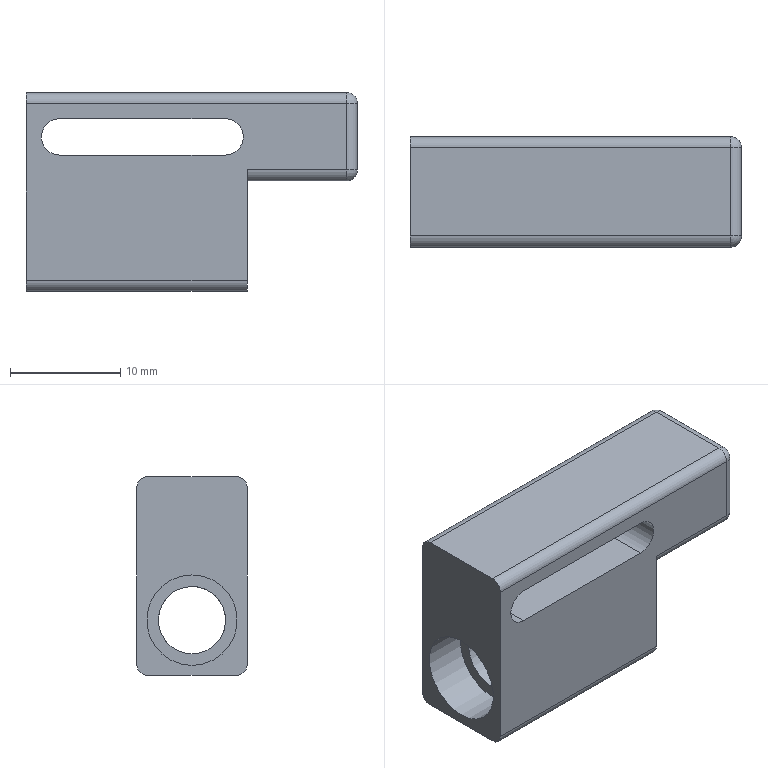CAM job | NX | 3+2 milling, drilling | part box 30 x 10 x 18 mm | stock box 35 x 12 x 23 mm
Tools:
number,name,description,diameter,corner_radius,flute_length,length,flutes
4,D4,平底铣刀-粗,4.0,0.0,25.0,75.0,2
9,D10,平底铣刀-粗,10.0,0.0,35.0,75.0,2
18,D4-J,平底铣刀-精,4.0,0.0,50.0,75.0,2
10,D10-J,平底铣刀-精,10.0,0.0,35.0,75.0,2
19,D6R0.5,圆鼻刀-粗,6.0,0.5,50.0,75.0,2
1,D80R0.8飞刀,圆鼻刀-粗,80.0,0.8,50.0,75.0,2
2,D6倒角刀,倒角刀,6.0,0.0,3.0,25.0,2
17,ZT6,钻头,6.0,0.0,35.0,50.0,2
Operations:
program,operation,operation_type,tool,method,geometry_group,spindle_rpm,surface_speed,feed_per_tooth,feed_cut,feed_plunge,cut_length_mm,path_length_mm,cut_time_min,machine_time_min
B,底壁铣飞面一刀开粗_COPY,VolumeBased25DMillingOperation,D10,分层开粗-切深K-步距G,W-B,7000.0,219.911,0.2143,3000.0,100.0,807.18,888.751,0.2691,0.2772
B,底壁铣分层开粗-中_COPY,VolumeBased25DMillingOperation,D10,分层开粗-切深K-步距G,W-B,7000.0,219.911,0.2857,4000.0,100.0,1176.861,1411.293,0.2942,0.3177
B,等高螺旋爬面_COPY,ZLevelMilling,D6R0.5,等高爬面-切深K-步距G,W-B,7000.0,175.929,0.3214,4500.0,100.0,1234.874,1273.374,0.2744,0.2783
B,平面去毛刺6X45L_COPY,SurfaceContour,D6倒角刀,爬面_倒角-切深0-步距G,W-B,6500.0,122.519,0.1154,1500.0,100.0,78.519,133.831,0.0523,0.0579
B,底壁铣飞面一刀精光_COPY,VolumeBased25DMillingOperation,D10-J,侧刃精光-切深K-步距G,W-B,7000.0,219.911,0.0714,1000.0,100.0,89.149,125.149,0.0891,0.0927
B,底壁铣精光底面-中_COPY,VolumeBased25DMillingOperation,D10-J,精光步距切深关,W-B,8000.0,251.32,0.0625,1000.0,100.0,49.923,96.523,0.0499,0.0546
B,底壁铣精光侧面-中-选底面_COPY_1,VolumeBased25DMillingOperation,D10-J,侧刃精光-切深K-步距G,W-B,8000.0,251.32,0.0625,1000.0,100.0,35.035,82.635,0.035,0.0398
A,顶面,FaceMilling,D80R0.8飞刀,侧刃精光-切深K-步距G,W-A,5000.0,1256.637,0.1,1000.0,100.0,112.0,148.0,0.112,0.1156
A,外形粗_2,VolumeBased25DMillingOperation,D10,METHOD,W-A,8000.0,251.327,0.3125,5000.0,80.0,3454.737,3523.437,0.6909,0.6978
A,沉头孔打点-深0.8,Operation,D6倒角刀,NONE,W-A,8000.0,150.796,0.0312,500.0,90.0,1.8,43.6,0.0036,0.0078
A,沉头孔-钻孔0段,Operation,ZT6,NONE,W-A,2800.0,53.658,0.0357,200.0,90.0,24.803,89.605,0.124,0.1305
A,铣孔开粗D4_1,CylinderMilling,D4,NONE,W-A,8000.0,100.531,0.075,1200.0,100.0,207.399,250.899,0.1728,0.1772
A,仅选体,SurfaceContour,D6倒角刀,METHOD,W-A,8000.0,150.796,0.1875,3000.0,100.0,71.598,107.399,0.0239,0.0274
A,铣倒角_1,PlanarMilling,D6倒角刀,NONE,W-A,8000.0,150.796,0.0312,500.0,100.0,34.596,70.596,0.0692,0.0728
A,底壁铣精光侧面-中-选底面_COPY,VolumeBased25DMillingOperation,D4-J,侧刃精光-切深K-步距G,W-A,6000.0,75.398,0.0417,500.0,100.0,19.145,45.545,0.0383,0.0409
A,底壁铣精光侧面-中_COPY,VolumeBased25DMillingOperation,D4-J,侧刃精光-切深K-步距G,W-A,6000.0,75.398,0.025,300.0,100.0,50.259,108.509,0.1675,0.1734
A,外形半精_2,VolumeBased25DMillingOperation,D10-J,METHOD,W-A,8000.0,251.327,0.0625,1000.0,100.0,181.338,352.451,0.1813,0.1984